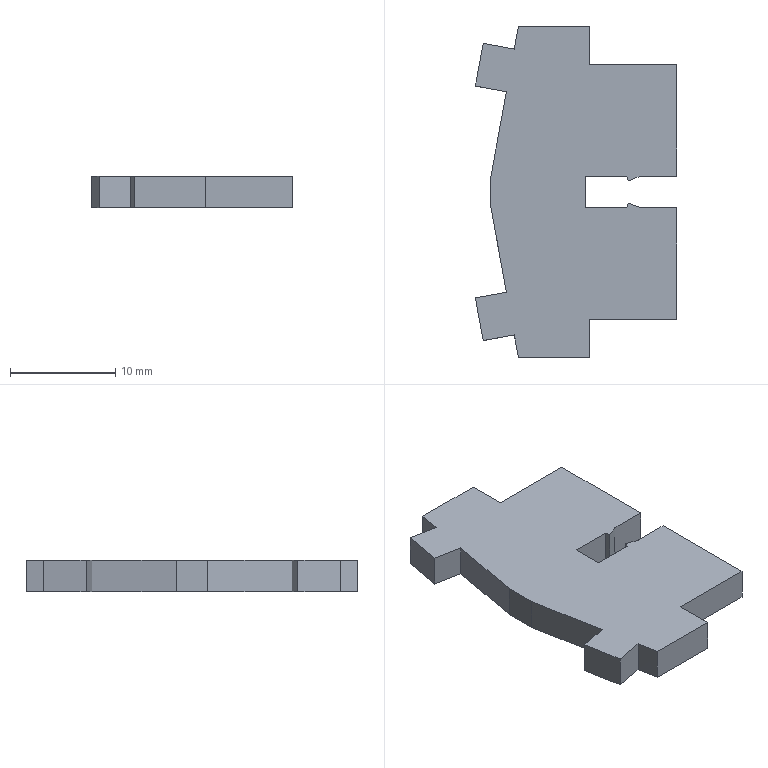Part | SolidWorks | features BaseBody 1 | 1 solid | 30 faces | box 19.083 x 31.429 x 3 mm | volume 1367 mm3 | plane 28 | spline 2
STEP:
#1=CARTESIAN_POINT('',(8.255,-1.366,-1.5));
#2=VERTEX_POINT('',#1);
#3=CARTESIAN_POINT('',(11.71,-1.366,-1.5));
#4=VERTEX_POINT('',#3);
#5=CARTESIAN_POINT('',(8.255,-1.366,-1.5));
#6=DIRECTION('',(1.,0.,0.));
#7=VECTOR('',#6,1000.);
#8=LINE('',#5,#7);
#9=EDGE_CURVE('',#2,#4,#8,.T.);
#10=ORIENTED_EDGE('',*,*,#9,.T.);
#11=CARTESIAN_POINT('',(11.71,-11.952,-1.5));
#12=VERTEX_POINT('',#11);
#13=CARTESIAN_POINT('',(11.71,-1.366,-1.5));
#14=DIRECTION('',(0.,-1.,0.));
#15=VECTOR('',#14,1000.);
#16=LINE('',#13,#15);
#17=EDGE_CURVE('',#4,#12,#16,.T.);
#18=ORIENTED_EDGE('',*,*,#17,.T.);
#19=CARTESIAN_POINT('',(3.461,-11.952,-1.5));
#20=VERTEX_POINT('',#19);
#21=CARTESIAN_POINT('',(11.71,-11.952,-1.5));
#22=DIRECTION('',(-1.,0.,0.));
#23=VECTOR('',#22,1000.);
#24=LINE('',#21,#23);
#25=EDGE_CURVE('',#12,#20,#24,.T.);
#26=ORIENTED_EDGE('',*,*,#25,.T.);
#27=CARTESIAN_POINT('',(3.461,-15.582,-1.5));
#28=VERTEX_POINT('',#27);
#29=CARTESIAN_POINT('',(3.461,-11.952,-1.5));
#30=DIRECTION('',(0.,-1.,0.));
#31=VECTOR('',#30,1000.);
#32=LINE('',#29,#31);
#33=EDGE_CURVE('',#20,#28,#32,.T.);
#34=ORIENTED_EDGE('',*,*,#33,.T.);
#35=CARTESIAN_POINT('',(-3.282,-15.582,-1.5));
#36=VERTEX_POINT('',#35);
#37=CARTESIAN_POINT('',(3.461,-15.582,-1.5));
#38=DIRECTION('',(-1.,0.,0.));
#39=VECTOR('',#38,1000.);
#40=LINE('',#37,#39);
#41=EDGE_CURVE('',#28,#36,#40,.T.);
#42=ORIENTED_EDGE('',*,*,#41,.T.);
#43=CARTESIAN_POINT('',(-3.684,-13.409,-1.5));
#44=VERTEX_POINT('',#43);
#45=CARTESIAN_POINT('',(-3.282,-15.582,-1.5));
#46=CARTESIAN_POINT('',(-3.415,-14.856,-1.5));
#47=CARTESIAN_POINT('',(-3.684,-13.409,-1.5));
#48=B_SPLINE_CURVE_WITH_KNOTS('',2,(#45,#46,#47),.UNSPECIFIED.,.F.,.F.,(3,3),(0.7576,0.7879),.UNSPECIFIED.);
#49=EDGE_CURVE('',#36,#44,#48,.T.);
#50=ORIENTED_EDGE('',*,*,#49,.T.);
#51=CARTESIAN_POINT('',(-6.629,-13.951,-1.5));
#52=VERTEX_POINT('',#51);
#53=CARTESIAN_POINT('',(-3.684,-13.409,-1.5));
#54=DIRECTION('',(-0.9835,-0.181,0.));
#55=VECTOR('',#54,1000.);
#56=LINE('',#53,#55);
#57=EDGE_CURVE('',#44,#52,#56,.T.);
#58=ORIENTED_EDGE('',*,*,#57,.T.);
#59=CARTESIAN_POINT('',(-7.372,-9.906,-1.5));
#60=VERTEX_POINT('',#59);
#61=CARTESIAN_POINT('',(-6.629,-13.951,-1.5));
#62=DIRECTION('',(-0.1807,0.9835,0.));
#63=VECTOR('',#62,1000.);
#64=LINE('',#61,#63);
#65=EDGE_CURVE('',#52,#60,#64,.T.);
#66=ORIENTED_EDGE('',*,*,#65,.T.);
#67=CARTESIAN_POINT('',(-4.425,-9.365,-1.5));
#68=VERTEX_POINT('',#67);
#69=CARTESIAN_POINT('',(-4.425,-9.365,-1.5));
#70=DIRECTION('',(-0.9836,-0.1805,0.));
#71=VECTOR('',#70,1000.);
#72=LINE('',#69,#71);
#73=EDGE_CURVE('',#68,#60,#72,.T.);
#74=ORIENTED_EDGE('',*,*,#73,.F.);
#75=CARTESIAN_POINT('',(-5.896,-1.37,-1.5));
#76=VERTEX_POINT('',#75);
#77=CARTESIAN_POINT('',(-4.425,-9.365,-1.5));
#78=DIRECTION('',(-0.1809,0.9835,0.));
#79=VECTOR('',#78,1000.);
#80=LINE('',#77,#79);
#81=EDGE_CURVE('',#68,#76,#80,.T.);
#82=ORIENTED_EDGE('',*,*,#81,.T.);
#83=CARTESIAN_POINT('',(-5.896,1.637,-1.5));
#84=VERTEX_POINT('',#83);
#85=CARTESIAN_POINT('',(-5.896,-1.37,-1.5));
#86=DIRECTION('',(0.,1.,0.));
#87=VECTOR('',#86,1000.);
#88=LINE('',#85,#87);
#89=EDGE_CURVE('',#76,#84,#88,.T.);
#90=ORIENTED_EDGE('',*,*,#89,.T.);
#91=CARTESIAN_POINT('',(-4.425,9.63,-1.5));
#92=VERTEX_POINT('',#91);
#93=CARTESIAN_POINT('',(-5.896,1.637,-1.5));
#94=DIRECTION('',(0.181,0.9835,0.));
#95=VECTOR('',#94,1000.);
#96=LINE('',#93,#95);
#97=EDGE_CURVE('',#84,#92,#96,.T.);
#98=ORIENTED_EDGE('',*,*,#97,.T.);
#99=CARTESIAN_POINT('',(-7.372,10.173,-1.5));
#100=VERTEX_POINT('',#99);
#101=CARTESIAN_POINT('',(-7.372,10.173,-1.5));
#102=DIRECTION('',(0.9835,-0.1809,0.));
#103=VECTOR('',#102,1000.);
#104=LINE('',#101,#103);
#105=EDGE_CURVE('',#100,#92,#104,.T.);
#106=ORIENTED_EDGE('',*,*,#105,.F.);
#107=CARTESIAN_POINT('',(-6.629,14.217,-1.5));
#108=VERTEX_POINT('',#107);
#109=CARTESIAN_POINT('',(-7.372,10.173,-1.5));
#110=CARTESIAN_POINT('',(-7.372,10.173,-1.5));
#111=CARTESIAN_POINT('',(-6.629,14.217,-1.5));
#112=B_SPLINE_CURVE_WITH_KNOTS('',2,(#109,#110,#111),.UNSPECIFIED.,.F.,.F.,(3,3),(0.1212,0.1515),.UNSPECIFIED.);
#113=EDGE_CURVE('',#100,#108,#112,.T.);
#114=ORIENTED_EDGE('',*,*,#113,.T.);
#115=CARTESIAN_POINT('',(-3.684,13.674,-1.5));
#116=VERTEX_POINT('',#115);
#117=CARTESIAN_POINT('',(-3.684,13.674,-1.5));
#118=DIRECTION('',(-0.9835,0.1811,0.));
#119=VECTOR('',#118,1000.);
#120=LINE('',#117,#119);
#121=EDGE_CURVE('',#116,#108,#120,.T.);
#122=ORIENTED_EDGE('',*,*,#121,.F.);
#123=CARTESIAN_POINT('',(-3.282,15.847,-1.5));
#124=VERTEX_POINT('',#123);
#125=CARTESIAN_POINT('',(-3.684,13.674,-1.5));
#126=CARTESIAN_POINT('',(-3.684,13.674,-1.5));
#127=CARTESIAN_POINT('',(-3.415,15.123,-1.5));
#128=CARTESIAN_POINT('',(-3.282,15.847,-1.5));
#129=B_SPLINE_CURVE_WITH_KNOTS('',3,(#125,#126,#127,#128),.UNSPECIFIED.,.F.,.F.,(4,4),(0.2121,0.2424),.UNSPECIFIED.);
#130=EDGE_CURVE('',#116,#124,#129,.T.);
#131=ORIENTED_EDGE('',*,*,#130,.T.);
#132=CARTESIAN_POINT('',(3.461,15.847,-1.5));
#133=VERTEX_POINT('',#132);
#134=CARTESIAN_POINT('',(-3.282,15.847,-1.5));
#135=CARTESIAN_POINT('',(-3.282,15.847,-1.5));
#136=CARTESIAN_POINT('',(3.461,15.847,-1.5));
#137=B_SPLINE_CURVE_WITH_KNOTS('',2,(#134,#135,#136),.UNSPECIFIED.,.F.,.F.,(3,3),(0.2424,0.2727),.UNSPECIFIED.);
#138=EDGE_CURVE('',#124,#133,#137,.T.);
#139=ORIENTED_EDGE('',*,*,#138,.T.);
#140=CARTESIAN_POINT('',(3.461,12.217,-1.5));
#141=VERTEX_POINT('',#140);
#142=CARTESIAN_POINT('',(3.461,15.847,-1.5));
#143=CARTESIAN_POINT('',(3.461,15.847,-1.5));
#144=CARTESIAN_POINT('',(3.461,12.217,-1.5));
#145=B_SPLINE_CURVE_WITH_KNOTS('',2,(#142,#143,#144),.UNSPECIFIED.,.F.,.F.,(3,3),(0.2727,0.303),.UNSPECIFIED.);
#146=EDGE_CURVE('',#133,#141,#145,.T.);
#147=ORIENTED_EDGE('',*,*,#146,.T.);
#148=CARTESIAN_POINT('',(11.71,12.217,-1.5));
#149=VERTEX_POINT('',#148);
#150=CARTESIAN_POINT('',(3.461,12.217,-1.5));
#151=CARTESIAN_POINT('',(3.461,12.217,-1.5));
#152=CARTESIAN_POINT('',(11.71,12.217,-1.5));
#153=B_SPLINE_CURVE_WITH_KNOTS('',2,(#150,#151,#152),.UNSPECIFIED.,.F.,.F.,(3,3),(0.303,0.3333),.UNSPECIFIED.);
#154=EDGE_CURVE('',#141,#149,#153,.T.);
#155=ORIENTED_EDGE('',*,*,#154,.T.);
#156=CARTESIAN_POINT('',(11.71,1.631,-1.5));
#157=VERTEX_POINT('',#156);
#158=CARTESIAN_POINT('',(11.71,12.217,-1.5));
#159=CARTESIAN_POINT('',(11.71,12.217,-1.5));
#160=CARTESIAN_POINT('',(11.71,1.631,-1.5));
#161=B_SPLINE_CURVE_WITH_KNOTS('',2,(#158,#159,#160),.UNSPECIFIED.,.F.,.F.,(3,3),(0.3333,0.3636),.UNSPECIFIED.);
#162=EDGE_CURVE('',#149,#157,#161,.T.);
#163=ORIENTED_EDGE('',*,*,#162,.T.);
#164=CARTESIAN_POINT('',(8.255,1.631,-1.5));
#165=VERTEX_POINT('',#164);
#166=CARTESIAN_POINT('',(11.71,1.631,-1.5));
#167=CARTESIAN_POINT('',(11.71,1.631,-1.5));
#168=CARTESIAN_POINT('',(8.255,1.631,-1.5));
#169=B_SPLINE_CURVE_WITH_KNOTS('',2,(#166,#167,#168),.UNSPECIFIED.,.F.,.F.,(3,3),(0.3636,0.3939),.UNSPECIFIED.);
#170=EDGE_CURVE('',#157,#165,#169,.T.);
#171=ORIENTED_EDGE('',*,*,#170,.T.);
#172=CARTESIAN_POINT('',(7.128,1.181,-1.5));
#173=VERTEX_POINT('',#172);
#174=CARTESIAN_POINT('',(8.255,1.631,-1.5));
#175=CARTESIAN_POINT('',(8.255,1.631,-1.5));
#176=CARTESIAN_POINT('',(7.128,1.181,-1.5));
#177=B_SPLINE_CURVE_WITH_KNOTS('',2,(#174,#175,#176),.UNSPECIFIED.,.F.,.F.,(3,3),(0.3939,0.4242),.UNSPECIFIED.);
#178=EDGE_CURVE('',#165,#173,#177,.T.);
#179=ORIENTED_EDGE('',*,*,#178,.T.);
#180=CARTESIAN_POINT('',(7.001,1.631,-1.5));
#181=VERTEX_POINT('',#180);
#182=CARTESIAN_POINT('',(7.128,1.181,-1.5));
#183=CARTESIAN_POINT('',(7.128,1.181,-1.5));
#184=CARTESIAN_POINT('',(7.001,1.631,-1.5));
#185=B_SPLINE_CURVE_WITH_KNOTS('',2,(#182,#183,#184),.UNSPECIFIED.,.F.,.F.,(3,3),(0.4242,0.4545),.UNSPECIFIED.);
#186=EDGE_CURVE('',#173,#181,#185,.T.);
#187=ORIENTED_EDGE('',*,*,#186,.T.);
#188=CARTESIAN_POINT('',(3.082,1.631,-1.5));
#189=VERTEX_POINT('',#188);
#190=CARTESIAN_POINT('',(7.001,1.631,-1.5));
#191=CARTESIAN_POINT('',(7.001,1.631,-1.5));
#192=CARTESIAN_POINT('',(3.082,1.631,-1.5));
#193=B_SPLINE_CURVE_WITH_KNOTS('',2,(#190,#191,#192),.UNSPECIFIED.,.F.,.F.,(3,3),(0.4545,0.4848),.UNSPECIFIED.);
#194=EDGE_CURVE('',#181,#189,#193,.T.);
#195=ORIENTED_EDGE('',*,*,#194,.T.);
#196=CARTESIAN_POINT('',(3.082,-1.366,-1.5));
#197=VERTEX_POINT('',#196);
#198=CARTESIAN_POINT('',(3.082,1.631,-1.5));
#199=CARTESIAN_POINT('',(3.082,1.631,-1.5));
#200=CARTESIAN_POINT('',(3.082,-1.366,-1.5));
#201=B_SPLINE_CURVE_WITH_KNOTS('',2,(#198,#199,#200),.UNSPECIFIED.,.F.,.F.,(3,3),(0.4848,0.5152),.UNSPECIFIED.);
#202=EDGE_CURVE('',#189,#197,#201,.T.);
#203=ORIENTED_EDGE('',*,*,#202,.T.);
#204=CARTESIAN_POINT('',(7.001,-1.366,-1.5));
#205=VERTEX_POINT('',#204);
#206=CARTESIAN_POINT('',(3.082,-1.366,-1.5));
#207=DIRECTION('',(1.,0.,0.));
#208=VECTOR('',#207,1000.);
#209=LINE('',#206,#208);
#210=EDGE_CURVE('',#197,#205,#209,.T.);
#211=ORIENTED_EDGE('',*,*,#210,.T.);
#212=CARTESIAN_POINT('',(7.115,-0.9154,-1.5));
#213=VERTEX_POINT('',#212);
#214=CARTESIAN_POINT('',(7.001,-1.366,-1.5));
#215=DIRECTION('',(0.2459,0.9693,0.));
#216=VECTOR('',#215,1000.);
#217=LINE('',#214,#216);
#218=EDGE_CURVE('',#205,#213,#217,.T.);
#219=ORIENTED_EDGE('',*,*,#218,.T.);
#220=CARTESIAN_POINT('',(7.115,-0.9154,-1.5));
#221=DIRECTION('',(0.9299,-0.3678,0.));
#222=VECTOR('',#221,1000.);
#223=LINE('',#220,#222);
#224=EDGE_CURVE('',#213,#2,#223,.T.);
#225=ORIENTED_EDGE('',*,*,#224,.T.);
#226=EDGE_LOOP('',(#10,#18,#26,#34,#42,#50,#58,#66,#74,#82,#90,#98,#106,#114,#122,#131,#139,#147,#155,#163,#171,#179,#187,#195,#203,#211,#219,#225));
#227=FACE_OUTER_BOUND('',#226,.T.);
#228=CARTESIAN_POINT('',(-3.449,-14.676,-1.5));
#229=DIRECTION('',(0.,0.,-1.));
#230=DIRECTION('',(0.,-1.,0.));
#231=AXIS2_PLACEMENT_3D('',#228,#229,#230);
#232=PLANE('',#231);
#233=ADVANCED_FACE('',(#227),#232,.T.);
#234=CARTESIAN_POINT('',(8.255,-1.366,1.5));
#235=VERTEX_POINT('',#234);
#236=CARTESIAN_POINT('',(11.71,-1.366,1.5));
#237=VERTEX_POINT('',#236);
#238=CARTESIAN_POINT('',(8.255,-1.366,1.5));
#239=DIRECTION('',(1.,0.,0.));
#240=VECTOR('',#239,1000.);
#241=LINE('',#238,#240);
#242=EDGE_CURVE('',#235,#237,#241,.T.);
#243=ORIENTED_EDGE('',*,*,#242,.F.);
#244=CARTESIAN_POINT('',(7.115,-0.9154,1.5));
#245=VERTEX_POINT('',#244);
#246=CARTESIAN_POINT('',(7.115,-0.9154,1.5));
#247=DIRECTION('',(0.9299,-0.3678,0.));
#248=VECTOR('',#247,1000.);
#249=LINE('',#246,#248);
#250=EDGE_CURVE('',#245,#235,#249,.T.);
#251=ORIENTED_EDGE('',*,*,#250,.F.);
#252=CARTESIAN_POINT('',(7.001,-1.366,1.5));
#253=VERTEX_POINT('',#252);
#254=CARTESIAN_POINT('',(7.001,-1.366,1.5));
#255=DIRECTION('',(0.2459,0.9693,0.));
#256=VECTOR('',#255,1000.);
#257=LINE('',#254,#256);
#258=EDGE_CURVE('',#253,#245,#257,.T.);
#259=ORIENTED_EDGE('',*,*,#258,.F.);
#260=CARTESIAN_POINT('',(3.082,-1.366,1.5));
#261=VERTEX_POINT('',#260);
#262=CARTESIAN_POINT('',(3.082,-1.366,1.5));
#263=DIRECTION('',(1.,0.,0.));
#264=VECTOR('',#263,1000.);
#265=LINE('',#262,#264);
#266=EDGE_CURVE('',#261,#253,#265,.T.);
#267=ORIENTED_EDGE('',*,*,#266,.F.);
#268=CARTESIAN_POINT('',(3.082,1.631,1.5));
#269=VERTEX_POINT('',#268);
#270=CARTESIAN_POINT('',(3.082,1.631,1.5));
#271=CARTESIAN_POINT('',(3.082,1.631,1.5));
#272=CARTESIAN_POINT('',(3.082,-1.366,1.5));
#273=B_SPLINE_CURVE_WITH_KNOTS('',2,(#270,#271,#272),.UNSPECIFIED.,.F.,.F.,(3,3),(0.4848,0.5152),.UNSPECIFIED.);
#274=EDGE_CURVE('',#269,#261,#273,.T.);
#275=ORIENTED_EDGE('',*,*,#274,.F.);
#276=CARTESIAN_POINT('',(7.001,1.631,1.5));
#277=VERTEX_POINT('',#276);
#278=CARTESIAN_POINT('',(7.001,1.631,1.5));
#279=CARTESIAN_POINT('',(7.001,1.631,1.5));
#280=CARTESIAN_POINT('',(3.082,1.631,1.5));
#281=B_SPLINE_CURVE_WITH_KNOTS('',2,(#278,#279,#280),.UNSPECIFIED.,.F.,.F.,(3,3),(0.4545,0.4848),.UNSPECIFIED.);
#282=EDGE_CURVE('',#277,#269,#281,.T.);
#283=ORIENTED_EDGE('',*,*,#282,.F.);
#284=CARTESIAN_POINT('',(7.128,1.181,1.5));
#285=VERTEX_POINT('',#284);
#286=CARTESIAN_POINT('',(7.128,1.181,1.5));
#287=CARTESIAN_POINT('',(7.128,1.181,1.5));
#288=CARTESIAN_POINT('',(7.001,1.631,1.5));
#289=B_SPLINE_CURVE_WITH_KNOTS('',2,(#286,#287,#288),.UNSPECIFIED.,.F.,.F.,(3,3),(0.4242,0.4545),.UNSPECIFIED.);
#290=EDGE_CURVE('',#285,#277,#289,.T.);
#291=ORIENTED_EDGE('',*,*,#290,.F.);
#292=CARTESIAN_POINT('',(8.255,1.631,1.5));
#293=VERTEX_POINT('',#292);
#294=CARTESIAN_POINT('',(8.255,1.631,1.5));
#295=CARTESIAN_POINT('',(8.255,1.631,1.5));
#296=CARTESIAN_POINT('',(7.128,1.181,1.5));
#297=B_SPLINE_CURVE_WITH_KNOTS('',2,(#294,#295,#296),.UNSPECIFIED.,.F.,.F.,(3,3),(0.3939,0.4242),.UNSPECIFIED.);
#298=EDGE_CURVE('',#293,#285,#297,.T.);
#299=ORIENTED_EDGE('',*,*,#298,.F.);
#300=CARTESIAN_POINT('',(11.71,1.631,1.5));
#301=VERTEX_POINT('',#300);
#302=CARTESIAN_POINT('',(11.71,1.631,1.5));
#303=CARTESIAN_POINT('',(11.71,1.631,1.5));
#304=CARTESIAN_POINT('',(8.255,1.631,1.5));
#305=B_SPLINE_CURVE_WITH_KNOTS('',2,(#302,#303,#304),.UNSPECIFIED.,.F.,.F.,(3,3),(0.3636,0.3939),.UNSPECIFIED.);
#306=EDGE_CURVE('',#301,#293,#305,.T.);
#307=ORIENTED_EDGE('',*,*,#306,.F.);
#308=CARTESIAN_POINT('',(11.71,12.217,1.5));
#309=VERTEX_POINT('',#308);
#310=CARTESIAN_POINT('',(11.71,12.217,1.5));
#311=CARTESIAN_POINT('',(11.71,12.217,1.5));
#312=CARTESIAN_POINT('',(11.71,1.631,1.5));
#313=B_SPLINE_CURVE_WITH_KNOTS('',2,(#310,#311,#312),.UNSPECIFIED.,.F.,.F.,(3,3),(0.3333,0.3636),.UNSPECIFIED.);
#314=EDGE_CURVE('',#309,#301,#313,.T.);
#315=ORIENTED_EDGE('',*,*,#314,.F.);
#316=CARTESIAN_POINT('',(3.461,12.217,1.5));
#317=VERTEX_POINT('',#316);
#318=CARTESIAN_POINT('',(3.461,12.217,1.5));
#319=CARTESIAN_POINT('',(3.461,12.217,1.5));
#320=CARTESIAN_POINT('',(11.71,12.217,1.5));
#321=B_SPLINE_CURVE_WITH_KNOTS('',2,(#318,#319,#320),.UNSPECIFIED.,.F.,.F.,(3,3),(0.303,0.3333),.UNSPECIFIED.);
#322=EDGE_CURVE('',#317,#309,#321,.T.);
#323=ORIENTED_EDGE('',*,*,#322,.F.);
#324=CARTESIAN_POINT('',(3.461,15.847,1.5));
#325=VERTEX_POINT('',#324);
#326=CARTESIAN_POINT('',(3.461,15.847,1.5));
#327=CARTESIAN_POINT('',(3.461,15.847,1.5));
#328=CARTESIAN_POINT('',(3.461,12.217,1.5));
#329=B_SPLINE_CURVE_WITH_KNOTS('',2,(#326,#327,#328),.UNSPECIFIED.,.F.,.F.,(3,3),(0.2727,0.303),.UNSPECIFIED.);
#330=EDGE_CURVE('',#325,#317,#329,.T.);
#331=ORIENTED_EDGE('',*,*,#330,.F.);
#332=CARTESIAN_POINT('',(-3.282,15.847,1.5));
#333=VERTEX_POINT('',#332);
#334=CARTESIAN_POINT('',(-3.282,15.847,1.5));
#335=CARTESIAN_POINT('',(-3.282,15.847,1.5));
#336=CARTESIAN_POINT('',(3.461,15.847,1.5));
#337=B_SPLINE_CURVE_WITH_KNOTS('',2,(#334,#335,#336),.UNSPECIFIED.,.F.,.F.,(3,3),(0.2424,0.2727),.UNSPECIFIED.);
#338=EDGE_CURVE('',#333,#325,#337,.T.);
#339=ORIENTED_EDGE('',*,*,#338,.F.);
#340=CARTESIAN_POINT('',(-3.684,13.674,1.5));
#341=VERTEX_POINT('',#340);
#342=CARTESIAN_POINT('',(-3.684,13.674,1.5));
#343=CARTESIAN_POINT('',(-3.684,13.674,1.5));
#344=CARTESIAN_POINT('',(-3.415,15.123,1.5));
#345=CARTESIAN_POINT('',(-3.282,15.847,1.5));
#346=B_SPLINE_CURVE_WITH_KNOTS('',3,(#342,#343,#344,#345),.UNSPECIFIED.,.F.,.F.,(4,4),(0.2121,0.2424),.UNSPECIFIED.);
#347=EDGE_CURVE('',#341,#333,#346,.T.);
#348=ORIENTED_EDGE('',*,*,#347,.F.);
#349=CARTESIAN_POINT('',(-6.629,14.217,1.5));
#350=VERTEX_POINT('',#349);
#351=CARTESIAN_POINT('',(-3.684,13.674,1.5));
#352=DIRECTION('',(-0.9835,0.1811,0.));
#353=VECTOR('',#352,1000.);
#354=LINE('',#351,#353);
#355=EDGE_CURVE('',#341,#350,#354,.T.);
#356=ORIENTED_EDGE('',*,*,#355,.T.);
#357=CARTESIAN_POINT('',(-7.372,10.173,1.5));
#358=VERTEX_POINT('',#357);
#359=CARTESIAN_POINT('',(-7.372,10.173,1.5));
#360=CARTESIAN_POINT('',(-7.372,10.173,1.5));
#361=CARTESIAN_POINT('',(-6.629,14.217,1.5));
#362=B_SPLINE_CURVE_WITH_KNOTS('',2,(#359,#360,#361),.UNSPECIFIED.,.F.,.F.,(3,3),(0.1212,0.1515),.UNSPECIFIED.);
#363=EDGE_CURVE('',#358,#350,#362,.T.);
#364=ORIENTED_EDGE('',*,*,#363,.F.);
#365=CARTESIAN_POINT('',(-4.425,9.63,1.5));
#366=VERTEX_POINT('',#365);
#367=CARTESIAN_POINT('',(-7.372,10.173,1.5));
#368=DIRECTION('',(0.9835,-0.1809,0.));
#369=VECTOR('',#368,1000.);
#370=LINE('',#367,#369);
#371=EDGE_CURVE('',#358,#366,#370,.T.);
#372=ORIENTED_EDGE('',*,*,#371,.T.);
#373=CARTESIAN_POINT('',(-5.896,1.637,1.5));
#374=VERTEX_POINT('',#373);
#375=CARTESIAN_POINT('',(-5.896,1.637,1.5));
#376=DIRECTION('',(0.181,0.9835,0.));
#377=VECTOR('',#376,1000.);
#378=LINE('',#375,#377);
#379=EDGE_CURVE('',#374,#366,#378,.T.);
#380=ORIENTED_EDGE('',*,*,#379,.F.);
#381=CARTESIAN_POINT('',(-5.896,-1.37,1.5));
#382=VERTEX_POINT('',#381);
#383=CARTESIAN_POINT('',(-5.896,-1.37,1.5));
#384=DIRECTION('',(0.,1.,0.));
#385=VECTOR('',#384,1000.);
#386=LINE('',#383,#385);
#387=EDGE_CURVE('',#382,#374,#386,.T.);
#388=ORIENTED_EDGE('',*,*,#387,.F.);
#389=CARTESIAN_POINT('',(-4.425,-9.365,1.5));
#390=VERTEX_POINT('',#389);
#391=CARTESIAN_POINT('',(-4.425,-9.365,1.5));
#392=DIRECTION('',(-0.1809,0.9835,0.));
#393=VECTOR('',#392,1000.);
#394=LINE('',#391,#393);
#395=EDGE_CURVE('',#390,#382,#394,.T.);
#396=ORIENTED_EDGE('',*,*,#395,.F.);
#397=CARTESIAN_POINT('',(-7.372,-9.906,1.5));
#398=VERTEX_POINT('',#397);
#399=CARTESIAN_POINT('',(-4.425,-9.365,1.5));
#400=DIRECTION('',(-0.9836,-0.1805,0.));
#401=VECTOR('',#400,1000.);
#402=LINE('',#399,#401);
#403=EDGE_CURVE('',#390,#398,#402,.T.);
#404=ORIENTED_EDGE('',*,*,#403,.T.);
#405=CARTESIAN_POINT('',(-6.629,-13.951,1.5));
#406=VERTEX_POINT('',#405);
#407=CARTESIAN_POINT('',(-6.629,-13.951,1.5));
#408=DIRECTION('',(-0.1807,0.9835,0.));
#409=VECTOR('',#408,1000.);
#410=LINE('',#407,#409);
#411=EDGE_CURVE('',#406,#398,#410,.T.);
#412=ORIENTED_EDGE('',*,*,#411,.F.);
#413=CARTESIAN_POINT('',(-3.684,-13.409,1.5));
#414=VERTEX_POINT('',#413);
#415=CARTESIAN_POINT('',(-3.684,-13.409,1.5));
#416=DIRECTION('',(-0.9835,-0.181,0.));
#417=VECTOR('',#416,1000.);
#418=LINE('',#415,#417);
#419=EDGE_CURVE('',#414,#406,#418,.T.);
#420=ORIENTED_EDGE('',*,*,#419,.F.);
#421=CARTESIAN_POINT('',(-3.282,-15.582,1.5));
#422=VERTEX_POINT('',#421);
#423=CARTESIAN_POINT('',(-3.282,-15.582,1.5));
#424=CARTESIAN_POINT('',(-3.415,-14.856,1.5));
#425=CARTESIAN_POINT('',(-3.684,-13.409,1.5));
#426=B_SPLINE_CURVE_WITH_KNOTS('',2,(#423,#424,#425),.UNSPECIFIED.,.F.,.F.,(3,3),(0.7576,0.7879),.UNSPECIFIED.);
#427=EDGE_CURVE('',#422,#414,#426,.T.);
#428=ORIENTED_EDGE('',*,*,#427,.F.);
#429=CARTESIAN_POINT('',(3.461,-15.582,1.5));
#430=VERTEX_POINT('',#429);
#431=CARTESIAN_POINT('',(3.461,-15.582,1.5));
#432=DIRECTION('',(-1.,0.,0.));
#433=VECTOR('',#432,1000.);
#434=LINE('',#431,#433);
#435=EDGE_CURVE('',#430,#422,#434,.T.);
#436=ORIENTED_EDGE('',*,*,#435,.F.);
#437=CARTESIAN_POINT('',(3.461,-11.952,1.5));
#438=VERTEX_POINT('',#437);
#439=CARTESIAN_POINT('',(3.461,-11.952,1.5));
#440=DIRECTION('',(0.,-1.,0.));
#441=VECTOR('',#440,1000.);
#442=LINE('',#439,#441);
#443=EDGE_CURVE('',#438,#430,#442,.T.);
#444=ORIENTED_EDGE('',*,*,#443,.F.);
#445=CARTESIAN_POINT('',(11.71,-11.952,1.5));
#446=VERTEX_POINT('',#445);
#447=CARTESIAN_POINT('',(11.71,-11.952,1.5));
#448=DIRECTION('',(-1.,0.,0.));
#449=VECTOR('',#448,1000.);
#450=LINE('',#447,#449);
#451=EDGE_CURVE('',#446,#438,#450,.T.);
#452=ORIENTED_EDGE('',*,*,#451,.F.);
#453=CARTESIAN_POINT('',(11.71,-1.366,1.5));
#454=DIRECTION('',(0.,-1.,0.));
#455=VECTOR('',#454,1000.);
#456=LINE('',#453,#455);
#457=EDGE_CURVE('',#237,#446,#456,.T.);
#458=ORIENTED_EDGE('',*,*,#457,.F.);
#459=EDGE_LOOP('',(#243,#251,#259,#267,#275,#283,#291,#299,#307,#315,#323,#331,#339,#348,#356,#364,#372,#380,#388,#396,#404,#412,#420,#428,#436,#444,#452,#458));
#460=FACE_OUTER_BOUND('',#459,.T.);
#461=CARTESIAN_POINT('',(-3.449,-14.676,1.5));
#462=DIRECTION('',(0.,0.,-1.));
#463=DIRECTION('',(0.,-1.,0.));
#464=AXIS2_PLACEMENT_3D('',#461,#462,#463);
#465=PLANE('',#464);
#466=ADVANCED_FACE('',(#460),#465,.F.);
#467=ORIENTED_EDGE('',*,*,#17,.F.);
#468=CARTESIAN_POINT('',(11.71,-1.366,1.5));
#469=DIRECTION('',(0.,0.,-1.));
#470=VECTOR('',#469,1000.);
#471=LINE('',#468,#470);
#472=EDGE_CURVE('',#237,#4,#471,.T.);
#473=ORIENTED_EDGE('',*,*,#472,.F.);
#474=ORIENTED_EDGE('',*,*,#457,.T.);
#475=CARTESIAN_POINT('',(11.71,-11.952,1.5));
#476=DIRECTION('',(0.,0.,-1.));
#477=VECTOR('',#476,1000.);
#478=LINE('',#475,#477);
#479=EDGE_CURVE('',#446,#12,#478,.T.);
#480=ORIENTED_EDGE('',*,*,#479,.T.);
#481=EDGE_LOOP('',(#467,#473,#474,#480));
#482=FACE_OUTER_BOUND('',#481,.T.);
#483=CARTESIAN_POINT('',(11.71,-1.366,1.5));
#484=DIRECTION('',(1.,0.,0.));
#485=DIRECTION('',(0.,1.,0.));
#486=AXIS2_PLACEMENT_3D('',#483,#484,#485);
#487=PLANE('',#486);
#488=ADVANCED_FACE('',(#482),#487,.T.);
#489=ORIENTED_EDGE('',*,*,#25,.F.);
#490=ORIENTED_EDGE('',*,*,#479,.F.);
#491=ORIENTED_EDGE('',*,*,#451,.T.);
#492=CARTESIAN_POINT('',(3.461,-11.952,1.5));
#493=DIRECTION('',(0.,0.,-1.));
#494=VECTOR('',#493,1000.);
#495=LINE('',#492,#494);
#496=EDGE_CURVE('',#438,#20,#495,.T.);
#497=ORIENTED_EDGE('',*,*,#496,.T.);
#498=EDGE_LOOP('',(#489,#490,#491,#497));
#499=FACE_OUTER_BOUND('',#498,.T.);
#500=CARTESIAN_POINT('',(11.71,-11.952,1.5));
#501=DIRECTION('',(0.,-1.,0.));
#502=DIRECTION('',(0.,0.,-1.));
#503=AXIS2_PLACEMENT_3D('',#500,#501,#502);
#504=PLANE('',#503);
#505=ADVANCED_FACE('',(#499),#504,.T.);
#506=ORIENTED_EDGE('',*,*,#33,.F.);
#507=ORIENTED_EDGE('',*,*,#496,.F.);
#508=ORIENTED_EDGE('',*,*,#443,.T.);
#509=CARTESIAN_POINT('',(3.461,-15.582,1.5));
#510=DIRECTION('',(0.,0.,-1.));
#511=VECTOR('',#510,1000.);
#512=LINE('',#509,#511);
#513=EDGE_CURVE('',#430,#28,#512,.T.);
#514=ORIENTED_EDGE('',*,*,#513,.T.);
#515=EDGE_LOOP('',(#506,#507,#508,#514));
#516=FACE_OUTER_BOUND('',#515,.T.);
#517=CARTESIAN_POINT('',(3.461,-11.952,1.5));
#518=DIRECTION('',(1.,0.,0.));
#519=DIRECTION('',(0.,1.,0.));
#520=AXIS2_PLACEMENT_3D('',#517,#518,#519);
#521=PLANE('',#520);
#522=ADVANCED_FACE('',(#516),#521,.T.);
#523=ORIENTED_EDGE('',*,*,#41,.F.);
#524=ORIENTED_EDGE('',*,*,#513,.F.);
#525=ORIENTED_EDGE('',*,*,#435,.T.);
#526=CARTESIAN_POINT('',(-3.282,-15.582,1.5));
#527=DIRECTION('',(0.,0.,-1.));
#528=VECTOR('',#527,1000.);
#529=LINE('',#526,#528);
#530=EDGE_CURVE('',#422,#36,#529,.T.);
#531=ORIENTED_EDGE('',*,*,#530,.T.);
#532=EDGE_LOOP('',(#523,#524,#525,#531));
#533=FACE_OUTER_BOUND('',#532,.T.);
#534=CARTESIAN_POINT('',(3.461,-15.582,1.5));
#535=DIRECTION('',(0.,-1.,0.));
#536=DIRECTION('',(0.,0.,-1.));
#537=AXIS2_PLACEMENT_3D('',#534,#535,#536);
#538=PLANE('',#537);
#539=ADVANCED_FACE('',(#533),#538,.T.);
#540=ORIENTED_EDGE('',*,*,#49,.F.);
#541=ORIENTED_EDGE('',*,*,#530,.F.);
#542=ORIENTED_EDGE('',*,*,#427,.T.);
#543=CARTESIAN_POINT('',(-3.684,-13.409,1.5));
#544=DIRECTION('',(0.,0.,-1.));
#545=VECTOR('',#544,1000.);
#546=LINE('',#543,#545);
#547=EDGE_CURVE('',#414,#44,#546,.T.);
#548=ORIENTED_EDGE('',*,*,#547,.T.);
#549=EDGE_LOOP('',(#540,#541,#542,#548));
#550=FACE_OUTER_BOUND('',#549,.T.);
#551=CARTESIAN_POINT('',(-3.282,-15.582,1.5));
#552=CARTESIAN_POINT('',(-3.282,-15.582,-1.5));
#553=CARTESIAN_POINT('',(-3.415,-14.856,1.5));
#554=CARTESIAN_POINT('',(-3.415,-14.856,-1.5));
#555=CARTESIAN_POINT('',(-3.684,-13.409,1.5));
#556=CARTESIAN_POINT('',(-3.684,-13.409,-1.5));
#557=B_SPLINE_SURFACE_WITH_KNOTS('',2,1,((#551,#552),(#553,#554),(#555,#556)),.UNSPECIFIED.,.F.,.F.,.F.,(3,3),(2,2),(0.7576,0.7879),(0.,1.),.UNSPECIFIED.);
#558=ADVANCED_FACE('',(#550),#557,.T.);
#559=ORIENTED_EDGE('',*,*,#57,.F.);
#560=ORIENTED_EDGE('',*,*,#547,.F.);
#561=ORIENTED_EDGE('',*,*,#419,.T.);
#562=CARTESIAN_POINT('',(-6.629,-13.951,1.5));
#563=DIRECTION('',(0.,0.,-1.));
#564=VECTOR('',#563,1000.);
#565=LINE('',#562,#564);
#566=EDGE_CURVE('',#406,#52,#565,.T.);
#567=ORIENTED_EDGE('',*,*,#566,.T.);
#568=EDGE_LOOP('',(#559,#560,#561,#567));
#569=FACE_OUTER_BOUND('',#568,.T.);
#570=CARTESIAN_POINT('',(-3.684,-13.409,1.5));
#571=DIRECTION('',(0.181,-0.9835,0.));
#572=DIRECTION('',(0.,0.,-1.));
#573=AXIS2_PLACEMENT_3D('',#570,#571,#572);
#574=PLANE('',#573);
#575=ADVANCED_FACE('',(#569),#574,.T.);
#576=ORIENTED_EDGE('',*,*,#65,.F.);
#577=ORIENTED_EDGE('',*,*,#566,.F.);
#578=ORIENTED_EDGE('',*,*,#411,.T.);
#579=CARTESIAN_POINT('',(-7.372,-9.906,1.5));
#580=DIRECTION('',(0.,0.,-1.));
#581=VECTOR('',#580,1000.);
#582=LINE('',#579,#581);
#583=EDGE_CURVE('',#398,#60,#582,.T.);
#584=ORIENTED_EDGE('',*,*,#583,.T.);
#585=EDGE_LOOP('',(#576,#577,#578,#584));
#586=FACE_OUTER_BOUND('',#585,.T.);
#587=CARTESIAN_POINT('',(-6.629,-13.951,1.5));
#588=DIRECTION('',(-0.9835,-0.1807,0.));
#589=DIRECTION('',(-0.1807,0.9835,0.));
#590=AXIS2_PLACEMENT_3D('',#587,#588,#589);
#591=PLANE('',#590);
#592=ADVANCED_FACE('',(#586),#591,.T.);
#593=ORIENTED_EDGE('',*,*,#73,.T.);
#594=ORIENTED_EDGE('',*,*,#583,.F.);
#595=ORIENTED_EDGE('',*,*,#403,.F.);
#596=CARTESIAN_POINT('',(-4.425,-9.365,1.5));
#597=DIRECTION('',(0.,0.,-1.));
#598=VECTOR('',#597,1000.);
#599=LINE('',#596,#598);
#600=EDGE_CURVE('',#390,#68,#599,.T.);
#601=ORIENTED_EDGE('',*,*,#600,.T.);
#602=EDGE_LOOP('',(#593,#594,#595,#601));
#603=FACE_OUTER_BOUND('',#602,.T.);
#604=CARTESIAN_POINT('',(-4.425,-9.365,1.5));
#605=DIRECTION('',(0.1805,-0.9836,0.));
#606=DIRECTION('',(0.,0.,-1.));
#607=AXIS2_PLACEMENT_3D('',#604,#605,#606);
#608=PLANE('',#607);
#609=ADVANCED_FACE('',(#603),#608,.F.);
#610=ORIENTED_EDGE('',*,*,#81,.F.);
#611=ORIENTED_EDGE('',*,*,#600,.F.);
#612=ORIENTED_EDGE('',*,*,#395,.T.);
#613=CARTESIAN_POINT('',(-5.896,-1.37,1.5));
#614=DIRECTION('',(0.,0.,-1.));
#615=VECTOR('',#614,1000.);
#616=LINE('',#613,#615);
#617=EDGE_CURVE('',#382,#76,#616,.T.);
#618=ORIENTED_EDGE('',*,*,#617,.T.);
#619=EDGE_LOOP('',(#610,#611,#612,#618));
#620=FACE_OUTER_BOUND('',#619,.T.);
#621=CARTESIAN_POINT('',(-4.425,-9.365,1.5));
#622=DIRECTION('',(-0.9835,-0.1809,0.));
#623=DIRECTION('',(-0.1809,0.9835,0.));
#624=AXIS2_PLACEMENT_3D('',#621,#622,#623);
#625=PLANE('',#624);
#626=ADVANCED_FACE('',(#620),#625,.T.);
#627=ORIENTED_EDGE('',*,*,#89,.F.);
#628=ORIENTED_EDGE('',*,*,#617,.F.);
#629=ORIENTED_EDGE('',*,*,#387,.T.);
#630=CARTESIAN_POINT('',(-5.896,1.637,1.5));
#631=DIRECTION('',(0.,0.,-1.));
#632=VECTOR('',#631,1000.);
#633=LINE('',#630,#632);
#634=EDGE_CURVE('',#374,#84,#633,.T.);
#635=ORIENTED_EDGE('',*,*,#634,.T.);
#636=EDGE_LOOP('',(#627,#628,#629,#635));
#637=FACE_OUTER_BOUND('',#636,.T.);
#638=CARTESIAN_POINT('',(-5.896,-1.37,1.5));
#639=DIRECTION('',(-1.,0.,0.));
#640=DIRECTION('',(0.,0.,1.));
#641=AXIS2_PLACEMENT_3D('',#638,#639,#640);
#642=PLANE('',#641);
#643=ADVANCED_FACE('',(#637),#642,.T.);
#644=ORIENTED_EDGE('',*,*,#97,.F.);
#645=ORIENTED_EDGE('',*,*,#634,.F.);
#646=ORIENTED_EDGE('',*,*,#379,.T.);
#647=CARTESIAN_POINT('',(-4.425,9.63,1.5));
#648=DIRECTION('',(0.,0.,-1.));
#649=VECTOR('',#648,1000.);
#650=LINE('',#647,#649);
#651=EDGE_CURVE('',#366,#92,#650,.T.);
#652=ORIENTED_EDGE('',*,*,#651,.T.);
#653=EDGE_LOOP('',(#644,#645,#646,#652));
#654=FACE_OUTER_BOUND('',#653,.T.);
#655=CARTESIAN_POINT('',(-5.896,1.637,1.5));
#656=DIRECTION('',(-0.9835,0.181,0.));
#657=DIRECTION('',(0.,0.,1.));
#658=AXIS2_PLACEMENT_3D('',#655,#656,#657);
#659=PLANE('',#658);
#660=ADVANCED_FACE('',(#654),#659,.T.);
#661=ORIENTED_EDGE('',*,*,#105,.T.);
#662=ORIENTED_EDGE('',*,*,#651,.F.);
#663=ORIENTED_EDGE('',*,*,#371,.F.);
#664=CARTESIAN_POINT('',(-7.372,10.173,1.5));
#665=DIRECTION('',(0.,0.,-1.));
#666=VECTOR('',#665,1000.);
#667=LINE('',#664,#666);
#668=EDGE_CURVE('',#358,#100,#667,.T.);
#669=ORIENTED_EDGE('',*,*,#668,.T.);
#670=EDGE_LOOP('',(#661,#662,#663,#669));
#671=FACE_OUTER_BOUND('',#670,.T.);
#672=CARTESIAN_POINT('',(-7.372,10.173,1.5));
#673=DIRECTION('',(0.1809,0.9835,0.));
#674=DIRECTION('',(0.,0.,-1.));
#675=AXIS2_PLACEMENT_3D('',#672,#673,#674);
#676=PLANE('',#675);
#677=ADVANCED_FACE('',(#671),#676,.F.);
#678=ORIENTED_EDGE('',*,*,#113,.F.);
#679=ORIENTED_EDGE('',*,*,#668,.F.);
#680=ORIENTED_EDGE('',*,*,#363,.T.);
#681=CARTESIAN_POINT('',(-6.629,14.217,1.5));
#682=DIRECTION('',(0.,0.,-1.));
#683=VECTOR('',#682,1000.);
#684=LINE('',#681,#683);
#685=EDGE_CURVE('',#350,#108,#684,.T.);
#686=ORIENTED_EDGE('',*,*,#685,.T.);
#687=EDGE_LOOP('',(#678,#679,#680,#686));
#688=FACE_OUTER_BOUND('',#687,.T.);
#689=CARTESIAN_POINT('',(-7.372,10.173,1.5));
#690=DIRECTION('',(-0.9835,0.1807,0.));
#691=DIRECTION('',(0.,0.,1.));
#692=AXIS2_PLACEMENT_3D('',#689,#690,#691);
#693=PLANE('',#692);
#694=ADVANCED_FACE('',(#688),#693,.T.);
#695=ORIENTED_EDGE('',*,*,#121,.T.);
#696=ORIENTED_EDGE('',*,*,#685,.F.);
#697=ORIENTED_EDGE('',*,*,#355,.F.);
#698=CARTESIAN_POINT('',(-3.684,13.674,1.5));
#699=DIRECTION('',(0.,0.,-1.));
#700=VECTOR('',#699,1000.);
#701=LINE('',#698,#700);
#702=EDGE_CURVE('',#341,#116,#701,.T.);
#703=ORIENTED_EDGE('',*,*,#702,.T.);
#704=EDGE_LOOP('',(#695,#696,#697,#703));
#705=FACE_OUTER_BOUND('',#704,.T.);
#706=CARTESIAN_POINT('',(-3.684,13.674,1.5));
#707=DIRECTION('',(-0.1811,-0.9835,0.));
#708=DIRECTION('',(-0.9835,0.1811,0.));
#709=AXIS2_PLACEMENT_3D('',#706,#707,#708);
#710=PLANE('',#709);
#711=ADVANCED_FACE('',(#705),#710,.F.);
#712=ORIENTED_EDGE('',*,*,#130,.F.);
#713=ORIENTED_EDGE('',*,*,#702,.F.);
#714=ORIENTED_EDGE('',*,*,#347,.T.);
#715=CARTESIAN_POINT('',(-3.282,15.847,1.5));
#716=DIRECTION('',(0.,0.,-1.));
#717=VECTOR('',#716,1000.);
#718=LINE('',#715,#717);
#719=EDGE_CURVE('',#333,#124,#718,.T.);
#720=ORIENTED_EDGE('',*,*,#719,.T.);
#721=EDGE_LOOP('',(#712,#713,#714,#720));
#722=FACE_OUTER_BOUND('',#721,.T.);
#723=CARTESIAN_POINT('',(-3.684,13.674,1.5));
#724=CARTESIAN_POINT('',(-3.684,13.674,-1.5));
#725=CARTESIAN_POINT('',(-3.684,13.674,1.5));
#726=CARTESIAN_POINT('',(-3.684,13.674,-1.5));
#727=CARTESIAN_POINT('',(-3.415,15.123,1.5));
#728=CARTESIAN_POINT('',(-3.415,15.123,-1.5));
#729=CARTESIAN_POINT('',(-3.282,15.847,1.5));
#730=CARTESIAN_POINT('',(-3.282,15.847,-1.5));
#731=B_SPLINE_SURFACE_WITH_KNOTS('',3,1,((#723,#724),(#725,#726),(#727,#728),(#729,#730)),.UNSPECIFIED.,.F.,.F.,.F.,(4,4),(2,2),(0.2121,0.2424),(0.,1.),.UNSPECIFIED.);
#732=ADVANCED_FACE('',(#722),#731,.T.);
#733=ORIENTED_EDGE('',*,*,#138,.F.);
#734=ORIENTED_EDGE('',*,*,#719,.F.);
#735=ORIENTED_EDGE('',*,*,#338,.T.);
#736=CARTESIAN_POINT('',(3.461,15.847,1.5));
#737=DIRECTION('',(0.,0.,-1.));
#738=VECTOR('',#737,1000.);
#739=LINE('',#736,#738);
#740=EDGE_CURVE('',#325,#133,#739,.T.);
#741=ORIENTED_EDGE('',*,*,#740,.T.);
#742=EDGE_LOOP('',(#733,#734,#735,#741));
#743=FACE_OUTER_BOUND('',#742,.T.);
#744=CARTESIAN_POINT('',(-3.282,15.847,1.5));
#745=DIRECTION('',(0.,1.,0.));
#746=DIRECTION('',(1.,0.,0.));
#747=AXIS2_PLACEMENT_3D('',#744,#745,#746);
#748=PLANE('',#747);
#749=ADVANCED_FACE('',(#743),#748,.T.);
#750=ORIENTED_EDGE('',*,*,#146,.F.);
#751=ORIENTED_EDGE('',*,*,#740,.F.);
#752=ORIENTED_EDGE('',*,*,#330,.T.);
#753=CARTESIAN_POINT('',(3.461,12.217,1.5));
#754=DIRECTION('',(0.,0.,-1.));
#755=VECTOR('',#754,1000.);
#756=LINE('',#753,#755);
#757=EDGE_CURVE('',#317,#141,#756,.T.);
#758=ORIENTED_EDGE('',*,*,#757,.T.);
#759=EDGE_LOOP('',(#750,#751,#752,#758));
#760=FACE_OUTER_BOUND('',#759,.T.);
#761=CARTESIAN_POINT('',(3.461,15.847,1.5));
#762=DIRECTION('',(1.,0.,0.));
#763=DIRECTION('',(0.,1.,0.));
#764=AXIS2_PLACEMENT_3D('',#761,#762,#763);
#765=PLANE('',#764);
#766=ADVANCED_FACE('',(#760),#765,.T.);
#767=ORIENTED_EDGE('',*,*,#154,.F.);
#768=ORIENTED_EDGE('',*,*,#757,.F.);
#769=ORIENTED_EDGE('',*,*,#322,.T.);
#770=CARTESIAN_POINT('',(11.71,12.217,1.5));
#771=DIRECTION('',(0.,0.,-1.));
#772=VECTOR('',#771,1000.);
#773=LINE('',#770,#772);
#774=EDGE_CURVE('',#309,#149,#773,.T.);
#775=ORIENTED_EDGE('',*,*,#774,.T.);
#776=EDGE_LOOP('',(#767,#768,#769,#775));
#777=FACE_OUTER_BOUND('',#776,.T.);
#778=CARTESIAN_POINT('',(3.461,12.217,1.5));
#779=DIRECTION('',(0.,1.,0.));
#780=DIRECTION('',(1.,0.,0.));
#781=AXIS2_PLACEMENT_3D('',#778,#779,#780);
#782=PLANE('',#781);
#783=ADVANCED_FACE('',(#777),#782,.T.);
#784=ORIENTED_EDGE('',*,*,#162,.F.);
#785=ORIENTED_EDGE('',*,*,#774,.F.);
#786=ORIENTED_EDGE('',*,*,#314,.T.);
#787=CARTESIAN_POINT('',(11.71,1.631,1.5));
#788=DIRECTION('',(0.,0.,-1.));
#789=VECTOR('',#788,1000.);
#790=LINE('',#787,#789);
#791=EDGE_CURVE('',#301,#157,#790,.T.);
#792=ORIENTED_EDGE('',*,*,#791,.T.);
#793=EDGE_LOOP('',(#784,#785,#786,#792));
#794=FACE_OUTER_BOUND('',#793,.T.);
#795=CARTESIAN_POINT('',(11.71,12.217,1.5));
#796=DIRECTION('',(1.,0.,0.));
#797=DIRECTION('',(0.,1.,0.));
#798=AXIS2_PLACEMENT_3D('',#795,#796,#797);
#799=PLANE('',#798);
#800=ADVANCED_FACE('',(#794),#799,.T.);
#801=ORIENTED_EDGE('',*,*,#170,.F.);
#802=ORIENTED_EDGE('',*,*,#791,.F.);
#803=ORIENTED_EDGE('',*,*,#306,.T.);
#804=CARTESIAN_POINT('',(8.255,1.631,1.5));
#805=DIRECTION('',(0.,0.,-1.));
#806=VECTOR('',#805,1000.);
#807=LINE('',#804,#806);
#808=EDGE_CURVE('',#293,#165,#807,.T.);
#809=ORIENTED_EDGE('',*,*,#808,.T.);
#810=EDGE_LOOP('',(#801,#802,#803,#809));
#811=FACE_OUTER_BOUND('',#810,.T.);
#812=CARTESIAN_POINT('',(11.71,1.631,1.5));
#813=DIRECTION('',(0.,-1.,0.));
#814=DIRECTION('',(0.,0.,-1.));
#815=AXIS2_PLACEMENT_3D('',#812,#813,#814);
#816=PLANE('',#815);
#817=ADVANCED_FACE('',(#811),#816,.T.);
#818=ORIENTED_EDGE('',*,*,#178,.F.);
#819=ORIENTED_EDGE('',*,*,#808,.F.);
#820=ORIENTED_EDGE('',*,*,#298,.T.);
#821=CARTESIAN_POINT('',(7.128,1.181,1.5));
#822=DIRECTION('',(0.,0.,-1.));
#823=VECTOR('',#822,1000.);
#824=LINE('',#821,#823);
#825=EDGE_CURVE('',#285,#173,#824,.T.);
#826=ORIENTED_EDGE('',*,*,#825,.T.);
#827=EDGE_LOOP('',(#818,#819,#820,#826));
#828=FACE_OUTER_BOUND('',#827,.T.);
#829=CARTESIAN_POINT('',(8.255,1.631,1.5));
#830=DIRECTION('',(0.3709,-0.9287,0.));
#831=DIRECTION('',(0.,0.,-1.));
#832=AXIS2_PLACEMENT_3D('',#829,#830,#831);
#833=PLANE('',#832);
#834=ADVANCED_FACE('',(#828),#833,.T.);
#835=ORIENTED_EDGE('',*,*,#186,.F.);
#836=ORIENTED_EDGE('',*,*,#825,.F.);
#837=ORIENTED_EDGE('',*,*,#290,.T.);
#838=CARTESIAN_POINT('',(7.001,1.631,1.5));
#839=DIRECTION('',(0.,0.,-1.));
#840=VECTOR('',#839,1000.);
#841=LINE('',#838,#840);
#842=EDGE_CURVE('',#277,#181,#841,.T.);
#843=ORIENTED_EDGE('',*,*,#842,.T.);
#844=EDGE_LOOP('',(#835,#836,#837,#843));
#845=FACE_OUTER_BOUND('',#844,.T.);
#846=CARTESIAN_POINT('',(7.128,1.181,1.5));
#847=DIRECTION('',(-0.9626,-0.271,0.));
#848=DIRECTION('',(-0.271,0.9626,0.));
#849=AXIS2_PLACEMENT_3D('',#846,#847,#848);
#850=PLANE('',#849);
#851=ADVANCED_FACE('',(#845),#850,.T.);
#852=ORIENTED_EDGE('',*,*,#194,.F.);
#853=ORIENTED_EDGE('',*,*,#842,.F.);
#854=ORIENTED_EDGE('',*,*,#282,.T.);
#855=CARTESIAN_POINT('',(3.082,1.631,1.5));
#856=DIRECTION('',(0.,0.,-1.));
#857=VECTOR('',#856,1000.);
#858=LINE('',#855,#857);
#859=EDGE_CURVE('',#269,#189,#858,.T.);
#860=ORIENTED_EDGE('',*,*,#859,.T.);
#861=EDGE_LOOP('',(#852,#853,#854,#860));
#862=FACE_OUTER_BOUND('',#861,.T.);
#863=CARTESIAN_POINT('',(7.001,1.631,1.5));
#864=DIRECTION('',(0.,-1.,0.));
#865=DIRECTION('',(0.,0.,-1.));
#866=AXIS2_PLACEMENT_3D('',#863,#864,#865);
#867=PLANE('',#866);
#868=ADVANCED_FACE('',(#862),#867,.T.);
#869=ORIENTED_EDGE('',*,*,#202,.F.);
#870=ORIENTED_EDGE('',*,*,#859,.F.);
#871=ORIENTED_EDGE('',*,*,#274,.T.);
#872=CARTESIAN_POINT('',(3.082,-1.366,1.5));
#873=DIRECTION('',(0.,0.,-1.));
#874=VECTOR('',#873,1000.);
#875=LINE('',#872,#874);
#876=EDGE_CURVE('',#261,#197,#875,.T.);
#877=ORIENTED_EDGE('',*,*,#876,.T.);
#878=EDGE_LOOP('',(#869,#870,#871,#877));
#879=FACE_OUTER_BOUND('',#878,.T.);
#880=CARTESIAN_POINT('',(3.082,1.631,1.5));
#881=DIRECTION('',(1.,0.,0.));
#882=DIRECTION('',(0.,1.,0.));
#883=AXIS2_PLACEMENT_3D('',#880,#881,#882);
#884=PLANE('',#883);
#885=ADVANCED_FACE('',(#879),#884,.T.);
#886=ORIENTED_EDGE('',*,*,#210,.F.);
#887=ORIENTED_EDGE('',*,*,#876,.F.);
#888=ORIENTED_EDGE('',*,*,#266,.T.);
#889=CARTESIAN_POINT('',(7.001,-1.366,1.5));
#890=DIRECTION('',(0.,0.,-1.));
#891=VECTOR('',#890,1000.);
#892=LINE('',#889,#891);
#893=EDGE_CURVE('',#253,#205,#892,.T.);
#894=ORIENTED_EDGE('',*,*,#893,.T.);
#895=EDGE_LOOP('',(#886,#887,#888,#894));
#896=FACE_OUTER_BOUND('',#895,.T.);
#897=CARTESIAN_POINT('',(3.082,-1.366,1.5));
#898=DIRECTION('',(0.,1.,0.));
#899=DIRECTION('',(1.,0.,0.));
#900=AXIS2_PLACEMENT_3D('',#897,#898,#899);
#901=PLANE('',#900);
#902=ADVANCED_FACE('',(#896),#901,.T.);
#903=ORIENTED_EDGE('',*,*,#218,.F.);
#904=ORIENTED_EDGE('',*,*,#893,.F.);
#905=ORIENTED_EDGE('',*,*,#258,.T.);
#906=CARTESIAN_POINT('',(7.115,-0.9154,1.5));
#907=DIRECTION('',(0.,0.,-1.));
#908=VECTOR('',#907,1000.);
#909=LINE('',#906,#908);
#910=EDGE_CURVE('',#245,#213,#909,.T.);
#911=ORIENTED_EDGE('',*,*,#910,.T.);
#912=EDGE_LOOP('',(#903,#904,#905,#911));
#913=FACE_OUTER_BOUND('',#912,.T.);
#914=CARTESIAN_POINT('',(7.001,-1.366,1.5));
#915=DIRECTION('',(-0.9693,0.2459,0.));
#916=DIRECTION('',(0.,0.,1.));
#917=AXIS2_PLACEMENT_3D('',#914,#915,#916);
#918=PLANE('',#917);
#919=ADVANCED_FACE('',(#913),#918,.T.);
#920=ORIENTED_EDGE('',*,*,#224,.F.);
#921=ORIENTED_EDGE('',*,*,#910,.F.);
#922=ORIENTED_EDGE('',*,*,#250,.T.);
#923=CARTESIAN_POINT('',(8.255,-1.366,1.5));
#924=DIRECTION('',(0.,0.,-1.));
#925=VECTOR('',#924,1000.);
#926=LINE('',#923,#925);
#927=EDGE_CURVE('',#235,#2,#926,.T.);
#928=ORIENTED_EDGE('',*,*,#927,.T.);
#929=EDGE_LOOP('',(#920,#921,#922,#928));
#930=FACE_OUTER_BOUND('',#929,.T.);
#931=CARTESIAN_POINT('',(7.115,-0.9154,1.5));
#932=DIRECTION('',(0.3678,0.9299,0.));
#933=DIRECTION('',(0.,0.,-1.));
#934=AXIS2_PLACEMENT_3D('',#931,#932,#933);
#935=PLANE('',#934);
#936=ADVANCED_FACE('',(#930),#935,.T.);
#937=ORIENTED_EDGE('',*,*,#9,.F.);
#938=ORIENTED_EDGE('',*,*,#927,.F.);
#939=ORIENTED_EDGE('',*,*,#242,.T.);
#940=ORIENTED_EDGE('',*,*,#472,.T.);
#941=EDGE_LOOP('',(#937,#938,#939,#940));
#942=FACE_OUTER_BOUND('',#941,.T.);
#943=CARTESIAN_POINT('',(8.255,-1.366,1.5));
#944=DIRECTION('',(0.,1.,0.));
#945=DIRECTION('',(1.,0.,0.));
#946=AXIS2_PLACEMENT_3D('',#943,#944,#945);
#947=PLANE('',#946);
#948=ADVANCED_FACE('',(#942),#947,.T.);
#949=CLOSED_SHELL('',(#233,#466,#488,#505,#522,#539,#558,#575,#592,#609,#626,#643,#660,#677,#694,#711,#732,#749,#766,#783,#800,#817,#834,#851,#868,#885,#902,#919,#936,#948));
#950=MANIFOLD_SOLID_BREP('',#949);
#951=CARTESIAN_POINT('',(0.,0.,0.));
#952=DIRECTION('',(0.,0.,1.));
#953=DIRECTION('',(1.,0.,0.));
#954=AXIS2_PLACEMENT_3D('',#951,#952,#953);
#955=(LENGTH_UNIT()NAMED_UNIT(*)SI_UNIT(.MILLI.,.METRE.));
#956=UNCERTAINTY_MEASURE_WITH_UNIT(LENGTH_MEASURE(0.00001),#955,'','');
#957=(NAMED_UNIT(*)PLANE_ANGLE_UNIT()SI_UNIT($,.RADIAN.));
#958=(NAMED_UNIT(*)SI_UNIT($,.STERADIAN.)SOLID_ANGLE_UNIT());
#959=(GEOMETRIC_REPRESENTATION_CONTEXT(3)GLOBAL_UNCERTAINTY_ASSIGNED_CONTEXT((#956))GLOBAL_UNIT_ASSIGNED_CONTEXT((#955,#957,#958))REPRESENTATION_CONTEXT('',''));
#960=ADVANCED_BREP_SHAPE_REPRESENTATION('',(#950,#954),#959);